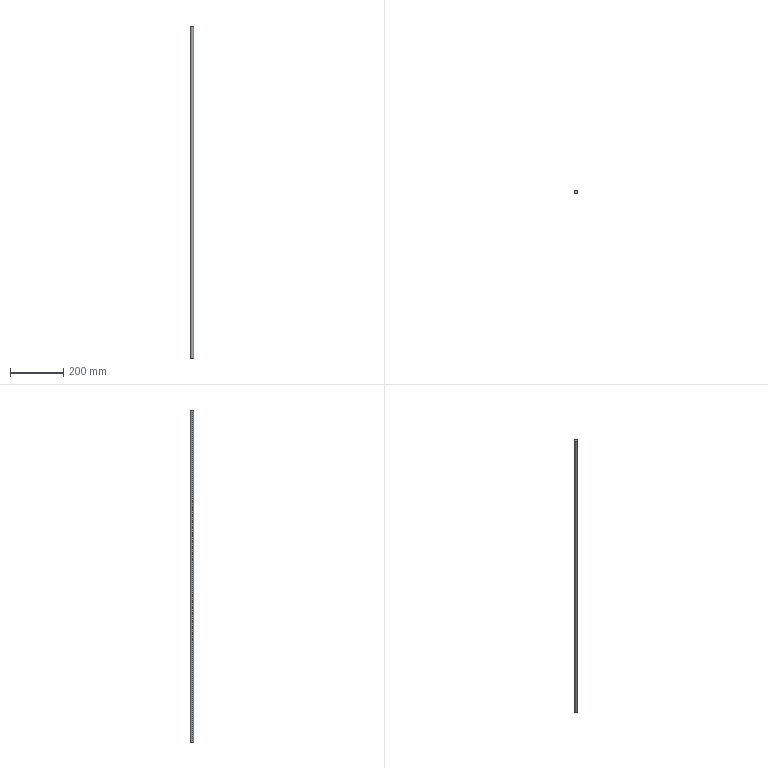Part | SolidWorks | features BaseBody 1 | 1 solid | 4 faces | box 12 x 12 x 1250 mm | volume 141372 mm3 | cylinder 2 | plane 2 | commonest cylinder face diameters 12 x2
STEP:
#1=CARTESIAN_POINT('',(-6.,0.,1250.));
#2=VERTEX_POINT('',#1);
#3=CARTESIAN_POINT('',(6.,0.,1250.));
#4=VERTEX_POINT('',#3);
#5=CARTESIAN_POINT('',(0.,0.,1250.));
#6=DIRECTION('',(0.,0.,-1.));
#7=DIRECTION('',(-1.,0.,0.));
#8=AXIS2_PLACEMENT_3D('',#5,#6,#7);
#9=CIRCLE('',#8,6.);
#10=EDGE_CURVE('',#2,#4,#9,.T.);
#11=ORIENTED_EDGE('',*,*,#10,.T.);
#12=CARTESIAN_POINT('',(6.,0.,0.));
#13=VERTEX_POINT('',#12);
#14=CARTESIAN_POINT('',(6.,0.,1250.));
#15=DIRECTION('',(0.,0.,-1.));
#16=VECTOR('',#15,1000.);
#17=LINE('',#14,#16);
#18=EDGE_CURVE('',#4,#13,#17,.T.);
#19=ORIENTED_EDGE('',*,*,#18,.T.);
#20=CARTESIAN_POINT('',(-6.,0.,0.));
#21=VERTEX_POINT('',#20);
#22=CARTESIAN_POINT('',(0.,0.,0.));
#23=DIRECTION('',(0.,0.,1.));
#24=DIRECTION('',(-1.,0.,0.));
#25=AXIS2_PLACEMENT_3D('',#22,#23,#24);
#26=CIRCLE('',#25,6.);
#27=EDGE_CURVE('',#13,#21,#26,.T.);
#28=ORIENTED_EDGE('',*,*,#27,.T.);
#29=CARTESIAN_POINT('',(-6.,0.,1250.));
#30=DIRECTION('',(0.,0.,-1.));
#31=VECTOR('',#30,1000.);
#32=LINE('',#29,#31);
#33=EDGE_CURVE('',#2,#21,#32,.T.);
#34=ORIENTED_EDGE('',*,*,#33,.F.);
#35=EDGE_LOOP('',(#11,#19,#28,#34));
#36=FACE_OUTER_BOUND('',#35,.T.);
#37=CARTESIAN_POINT('',(0.,0.,1250.));
#38=DIRECTION('',(0.,0.,-1.));
#39=DIRECTION('',(-1.,0.,0.));
#40=AXIS2_PLACEMENT_3D('',#37,#38,#39);
#41=CYLINDRICAL_SURFACE('',#40,6.);
#42=ADVANCED_FACE('',(#36),#41,.T.);
#43=ORIENTED_EDGE('',*,*,#18,.F.);
#44=CARTESIAN_POINT('',(0.,0.,1250.));
#45=DIRECTION('',(0.,0.,-1.));
#46=DIRECTION('',(-1.,0.,0.));
#47=AXIS2_PLACEMENT_3D('',#44,#45,#46);
#48=CIRCLE('',#47,6.);
#49=EDGE_CURVE('',#4,#2,#48,.T.);
#50=ORIENTED_EDGE('',*,*,#49,.T.);
#51=ORIENTED_EDGE('',*,*,#33,.T.);
#52=CARTESIAN_POINT('',(0.,0.,0.));
#53=DIRECTION('',(0.,0.,1.));
#54=DIRECTION('',(-1.,0.,0.));
#55=AXIS2_PLACEMENT_3D('',#52,#53,#54);
#56=CIRCLE('',#55,6.);
#57=EDGE_CURVE('',#21,#13,#56,.T.);
#58=ORIENTED_EDGE('',*,*,#57,.T.);
#59=EDGE_LOOP('',(#43,#50,#51,#58));
#60=FACE_OUTER_BOUND('',#59,.T.);
#61=CARTESIAN_POINT('',(0.,0.,1250.));
#62=DIRECTION('',(0.,0.,-1.));
#63=DIRECTION('',(-1.,0.,0.));
#64=AXIS2_PLACEMENT_3D('',#61,#62,#63);
#65=CYLINDRICAL_SURFACE('',#64,6.);
#66=ADVANCED_FACE('',(#60),#65,.T.);
#67=ORIENTED_EDGE('',*,*,#57,.F.);
#68=ORIENTED_EDGE('',*,*,#27,.F.);
#69=EDGE_LOOP('',(#67,#68));
#70=FACE_OUTER_BOUND('',#69,.T.);
#71=CARTESIAN_POINT('',(0.,0.,0.));
#72=DIRECTION('',(0.,0.,1.));
#73=DIRECTION('',(1.,0.,0.));
#74=AXIS2_PLACEMENT_3D('',#71,#72,#73);
#75=PLANE('',#74);
#76=ADVANCED_FACE('',(#70),#75,.F.);
#77=ORIENTED_EDGE('',*,*,#10,.F.);
#78=ORIENTED_EDGE('',*,*,#49,.F.);
#79=EDGE_LOOP('',(#77,#78));
#80=FACE_OUTER_BOUND('',#79,.T.);
#81=CARTESIAN_POINT('',(0.,0.,1250.));
#82=DIRECTION('',(0.,0.,1.));
#83=DIRECTION('',(1.,0.,0.));
#84=AXIS2_PLACEMENT_3D('',#81,#82,#83);
#85=PLANE('',#84);
#86=ADVANCED_FACE('',(#80),#85,.T.);
#87=CLOSED_SHELL('',(#42,#66,#76,#86));
#88=MANIFOLD_SOLID_BREP('',#87);
#89=CARTESIAN_POINT('',(0.,0.,0.));
#90=DIRECTION('',(0.,0.,1.));
#91=DIRECTION('',(1.,0.,0.));
#92=AXIS2_PLACEMENT_3D('',#89,#90,#91);
#93=(LENGTH_UNIT()NAMED_UNIT(*)SI_UNIT(.MILLI.,.METRE.));
#94=UNCERTAINTY_MEASURE_WITH_UNIT(LENGTH_MEASURE(0.00001),#93,'','');
#95=(NAMED_UNIT(*)PLANE_ANGLE_UNIT()SI_UNIT($,.RADIAN.));
#96=(NAMED_UNIT(*)SI_UNIT($,.STERADIAN.)SOLID_ANGLE_UNIT());
#97=(GEOMETRIC_REPRESENTATION_CONTEXT(3)GLOBAL_UNCERTAINTY_ASSIGNED_CONTEXT((#94))GLOBAL_UNIT_ASSIGNED_CONTEXT((#93,#95,#96))REPRESENTATION_CONTEXT('',''));
#98=ADVANCED_BREP_SHAPE_REPRESENTATION('',(#88,#92),#97);